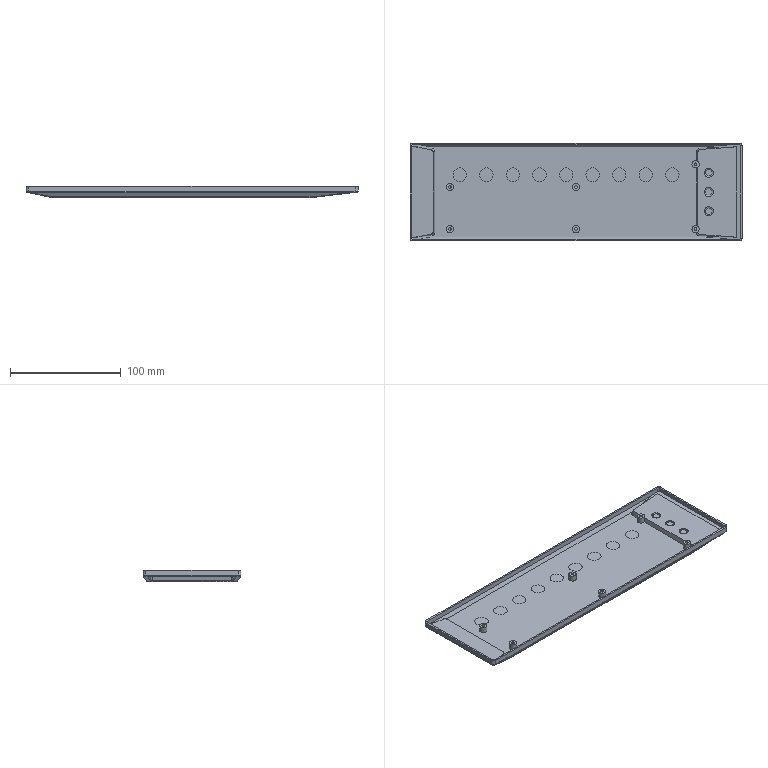NC program | NX | posted with a generic post | part box 300 x 88.5 x 10 mm
Lines 3382 to 4408 of 79950:
(FIXED_CONTOUR_COPY , TOOL : D3R0.5)
N6738 T09 M6
N6740 G54
N6742 G17 G0 G90 X-123.047 Y-18.46 S9500 M3
N6744 G43 Z30. H9
N6746 Z-1.2
N6748 G94 G1 Z-4.25 F1000.
N6750 G2 X-123.197 Y-18.2 R0.3
N6752 G1 Y-18.011 Z-4.267 F2500.
N6754 Y-17.674 Z-4.286
N6756 Y-17.336
N6758 Y-16.998 Z-4.267
N6760 Y-16.799 Z-4.25
N6762 X-123.161 Y-16.634 Z-4.246
N6764 Y-16.806 Z-4.269
N6766 Y-17.041 Z-4.288
N6768 Y-17.336 Z-4.305
N6770 Y-17.674
N6772 Y-18.011 Z-4.285
N6774 Y-18.238 Z-4.264
N6776 Y-18.367 Z-4.246
N6778 X-123.126 Y-18.498 Z-4.243
N6780 X-123.116 Y-18.526 Z-4.244
N6782 Y-18.256 Z-4.283
N6784 Y-18.167 Z-4.294
N6786 Y-17.923 Z-4.313
N6788 Y-17.674 Z-4.328
N6790 Y-17.336
N6792 Y-16.998 Z-4.308
N6794 Y-16.836 Z-4.294
N6796 Y-16.66 Z-4.272
N6798 Y-16.475 Z-4.244
N6800 X-123.055 Y-16.314 Z-4.248
N6802 Y-16.726 Z-4.31
N6804 Y-16.875 Z-4.328
N6806 Y-16.998 Z-4.338
N6808 Y-17.336 Z-4.358
N6810 Y-17.674
N6812 Y-18.011 Z-4.337
N6814 Y-18.129 Z-4.327
N6816 Y-18.349 Z-4.3
N6818 Y-18.689 Z-4.247
N6820 X-122.992 Y-18.829 Z-4.248
N6822 Y-18.687 Z-4.276
N6824 Y-18.349 Z-4.33
N6826 Y-18.09 Z-4.362
N6828 Y-17.799 Z-4.382
N6830 Y-17.674 Z-4.39
N6832 Y-17.336
N6834 Y-16.998 Z-4.369
N6836 Y-16.916 Z-4.362
N6838 Y-16.66 Z-4.331
N6840 Y-16.322 Z-4.278
N6842 Y-16.172 Z-4.248
N6844 X-122.925 Y-16.026 Z-4.25
N6846 Y-16.322 Z-4.309
N6848 Y-16.653 Z-4.363
N6850 Y-16.998 Z-4.403
N6852 Y-17.336 Z-4.424
N6854 Y-17.674
N6856 Y-18.048 Z-4.399
N6858 Y-18.349 Z-4.362
N6860 Y-18.687 Z-4.307
N6862 Y-18.976 Z-4.249
N6864 X-122.89 Y-19.049 Z-4.248
N6866 X-122.849 Y-19.117
N6868 Y-19.008 Z-4.276
N6870 Y-18.67 Z-4.345
N6872 Y-18.332 Z-4.401
N6874 Y-18.011 Z-4.44
N6876 Y-17.674 Z-4.462
N6878 Y-17.336
N6880 Y-16.998 Z-4.44
N6882 Y-16.66 Z-4.4
N6884 Y-16.322 Z-4.343
N6886 Y-15.984 Z-4.274
N6888 Y-15.879 Z-4.247
N6890 X-122.773 Y-15.748 Z-4.245
N6892 Y-15.984 Z-4.307
N6894 Y-16.078 Z-4.329
N6896 Y-16.416 Z-4.397
N6898 Y-16.66 Z-4.437
N6900 Y-16.998 Z-4.479
N6902 Y-17.336 Z-4.5
N6904 Y-17.674
N6906 Y-18.011 Z-4.478
N6908 Y-18.349 Z-4.436
N6910 Y-18.593 Z-4.395
N6912 Y-18.931 Z-4.327
N6914 Y-19.025 Z-4.304
N6916 Y-19.243 Z-4.248
N6918 X-122.692 Y-19.375 Z-4.247
N6920 Y-19.025 Z-4.339
N6922 Y-18.85 Z-4.381
N6924 Y-18.512 Z-4.448
N6926 Y-18.349 Z-4.475
N6928 Y-18.011 Z-4.518
N6930 Y-17.674 Z-4.541
N6932 Y-17.336
N6934 Y-16.998 Z-4.519
N6936 Y-16.66 Z-4.477
N6938 Y-16.497 Z-4.449
N6940 Y-16.159 Z-4.383
N6942 Y-15.984 Z-4.341
N6944 Y-15.646 Z-4.253
N6946 Y-15.626 Z-4.247
N6948 X-122.665 Y-15.586 Z-4.245
N6950 X-122.606 Y-15.511 Z-4.246
N6952 Y-15.646 Z-4.288
N6954 Y-15.984 Z-4.378
N6956 Y-16.246 Z-4.441
N6958 Y-16.584 Z-4.506
N6960 Y-16.66 Z-4.519
N6962 Y-16.998 Z-4.562
N6964 Y-17.336 Z-4.585
N6966 Y-17.674 Z-4.584
N6968 Y-18.011 Z-4.562
N6970 Y-18.349 Z-4.517
N6972 Y-18.426 Z-4.505
N6974 Y-18.764 Z-4.439
N6976 Y-19.025 Z-4.376
N6978 Y-19.363 Z-4.285
N6980 Y-19.488 Z-4.246
N6982 X-122.519 Y-19.598
N6984 Y-19.352 Z-4.324
N6986 Y-19.014 Z-4.416
N6988 Y-18.676 Z-4.497
N6990 Y-18.338 Z-4.561
N6992 Y-18.007 Z-4.605
N6994 Y-17.674 Z-4.628
N6996 Y-17.336
N6998 Y-16.998 Z-4.606
N7000 Y-16.66 Z-4.561
N7002 Y-16.322 Z-4.497
N7004 Y-15.984 Z-4.416
N7006 Y-15.657 Z-4.327
N7008 Y-15.401 Z-4.246
N7010 X-122.43 Y-15.291 Z-4.244
N7012 Y-15.746 Z-4.389
N7014 Y-16.084 Z-4.48
N7016 Y-16.322 Z-4.537
N7018 Y-16.422 Z-4.557
N7020 Y-16.66 Z-4.602
N7022 Y-16.998 Z-4.649
N7024 Y-17.336 Z-4.672
N7026 Y-17.674
N7028 Y-17.968 Z-4.652
N7030 Y-18.25 Z-4.616
N7032 Y-18.349 Z-4.601
N7034 Y-18.588 Z-4.555
N7036 Y-18.687 Z-4.535
N7038 Y-18.926 Z-4.477
N7040 Y-19.263 Z-4.386
N7042 Y-19.708 Z-4.245
N7044 X-122.402 Y-19.741 Z-4.243
N7046 X-122.341 Y-19.799 Z-4.244
N7048 Y-19.568 Z-4.325
N7050 Y-19.174 Z-4.449
N7052 Y-18.836 Z-4.539
N7054 Y-18.687 Z-4.575
N7056 Y-18.499 Z-4.614
N7058 Y-18.349 Z-4.643
N7060 Y-18.161 Z-4.671
N7062 Y-18.011 Z-4.691
N7064 Y-17.929 Z-4.7
N7066 Y-17.674 Z-4.716
N7068 Y-17.585 Z-4.718
N7070 Y-17.336 Z-4.717
N7072 Y-17.101 Z-4.702
N7074 Y-16.998 Z-4.692
N7076 Y-16.849 Z-4.672
N7078 Y-16.66 Z-4.644
N7080 Y-16.511 Z-4.616
N7082 Y-16.322 Z-4.577
N7084 Y-16.173 Z-4.541
N7086 Y-15.835 Z-4.451
N7088 Y-15.448 Z-4.33
N7090 Y-15.308 Z-4.282
N7092 Y-15.201 Z-4.244
N7094 X-122.252 Y-15.118 Z-4.245
N7096 Y-15.308 Z-4.314
N7098 Y-15.566 Z-4.402
N7100 Y-15.924 Z-4.514
N7102 Y-16.322 Z-4.617
N7104 Y-16.66 Z-4.686
N7106 Y-16.998 Z-4.735
N7108 Y-17.149 Z-4.749
N7110 Y-17.336 Z-4.761
N7112 Y-17.543 Z-4.763
N7114 Y-17.674 Z-4.761
N7116 Y-17.89 Z-4.747
N7118 Y-18.011 Z-4.734
N7120 Y-18.349 Z-4.684
N7122 Y-18.687 Z-4.615
N7124 Y-19.085 Z-4.511
N7126 Y-19.445 Z-4.398
N7128 Y-19.701 Z-4.311
N7130 Y-19.882 Z-4.245
N7132 X-122.163 Y-19.966 Z-4.246
N7134 Y-19.672 Z-4.353
N7136 Y-19.334 Z-4.469
N7138 Y-18.996 Z-4.574
N7140 Y-18.673 Z-4.658
N7142 Y-18.335 Z-4.729
N7144 Y-18.011 Z-4.777
N7146 Y-17.856 Z-4.793
N7148 Y-17.674 Z-4.805
N7150 Y-17.512 Z-4.808
N7152 Y-17.336 Z-4.805
N7154 Y-17.184 Z-4.796
N7156 Y-16.998 Z-4.779
N7158 Y-16.66 Z-4.728
N7160 Y-16.337 Z-4.66
N7162 Y-15.984 Z-4.568
N7164 Y-15.646 Z-4.462
N7166 Y-15.338 Z-4.357
N7168 Y-15.035 Z-4.246
N7170 X-122.087 Y-14.965
N7172 X-122.074 Y-14.955
N7174 Y-15.147 Z-4.318
N7176 Y-15.427 Z-4.42
N7178 Y-15.765 Z-4.535
N7180 Y-15.984 Z-4.603
N7182 Y-16.103 Z-4.638
N7184 Y-16.383 Z-4.711
N7186 Y-16.714 Z-4.78
N7188 Y-16.998 Z-4.822
N7190 Y-17.192 Z-4.841
N7192 Y-17.336 Z-4.85
N7194 Y-17.505 Z-4.853
N7196 Y-17.674 Z-4.849
N7198 Y-17.835 Z-4.84
N7200 Y-18.011 Z-4.821
N7202 Y-18.292 Z-4.778
N7204 Y-18.628 Z-4.708
N7206 Y-18.907 Z-4.635
N7208 Y-19.025 Z-4.6
N7210 Y-19.244 Z-4.532
N7212 Y-19.582 Z-4.417
N7214 Y-20.047 Z-4.246
N7216 X-122.02 Y-20.088 Z-4.245
N7218 X-121.985 Y-20.113
N7220 Y-19.888 Z-4.336
N7222 Y-19.493 Z-4.481
N7224 Y-19.155 Z-4.595
N7226 Y-19.025 Z-4.635
N7228 Y-18.817 Z-4.697
N7230 Y-18.584 Z-4.757
N7232 Y-18.249 Z-4.828
N7234 Y-18.011 Z-4.864
N7236 Y-17.791 Z-4.887
N7238 Y-17.674 Z-4.894
N7240 Y-17.498 Z-4.898
N7242 Y-17.336 Z-4.894
N7244 Y-17.178 Z-4.884
N7246 Y-16.998 Z-4.865
N7248 Y-16.755 Z-4.829
N7250 Y-16.429 Z-4.761
N7252 Y-16.192 Z-4.699
N7254 Y-15.984 Z-4.638
N7256 Y-15.854 Z-4.598
N7258 Y-15.516 Z-4.484
N7260 Y-15.127 Z-4.341
N7262 Y-14.887 Z-4.244
N7264 X-121.894 Y-14.825 Z-4.246
N7266 Y-15.279 Z-4.428
N7268 Y-15.646 Z-4.562
N7270 Y-15.984 Z-4.674
N7272 Y-16.283 Z-4.761
N7274 Y-16.475 Z-4.812
N7276 Y-16.66 Z-4.851
N7278 Y-16.796 Z-4.878
N7280 Y-16.943 Z-4.9
N7282 X-121.803 Y-16.703
N7284 Y-16.694
N7286 Y-16.526 Z-4.864
N7288 Y-16.322 Z-4.81
N7290 Y-15.998 Z-4.714
N7292 Y-15.698 Z-4.614
N7294 Y-15.36 Z-4.489
N7296 Y-14.821 Z-4.271
N7298 Y-14.764 Z-4.246
N7300 X-121.729 Y-14.716 Z-4.245
N7302 X-121.711 Y-14.705
N7304 Y-14.87 Z-4.317
N7306 Y-15.453 Z-4.555
N7308 Y-15.79 Z-4.679
N7310 Y-16.023 Z-4.758
N7312 Y-16.167 Z-4.804
N7314 Y-16.322 Z-4.849
N7316 Y-16.517 Z-4.9
N7318 X-121.618 Y-16.377
N7320 Y-16.368
N7322 Y-16.285 Z-4.877
N7324 Y-16.048 Z-4.801
N7326 Y-15.883 Z-4.745
N7328 Y-15.545 Z-4.62
N7330 Y-15.207 Z-4.483
N7332 Y-14.918 Z-4.363
N7334 Y-14.653 Z-4.248
N7336 X-121.525 Y-14.601 Z-4.247
N7338 Y-14.967 Z-4.41
N7340 Y-15.301 Z-4.549
N7342 Y-15.639 Z-4.687
N7344 Y-15.984 Z-4.814
N7346 Y-16.073 Z-4.846
N7348 Y-16.245 Z-4.9
N7350 X-121.431 Y-16.136
N7352 Y-16.132
N7354 Y-15.714 Z-4.746
N7356 Y-15.396 Z-4.615
N7358 Y-15.058 Z-4.473
N7360 Y-14.603 Z-4.269
N7362 Y-14.55 Z-4.244
N7364 X-121.394 Y-14.531 Z-4.243
N7366 X-121.335 Y-14.508 Z-4.245
N7368 Y-14.815 Z-4.387
N7370 Y-15.153 Z-4.538
N7372 Y-15.308 Z-4.602
N7374 Y-15.491 Z-4.682
N7376 Y-15.788 Z-4.804
N7378 Y-16.042 Z-4.9
N7380 X-121.24 Y-15.958
N7382 Y-15.863 Z-4.863
N7384 Y-15.587 Z-4.749
N7386 Y-15.249 Z-4.603
N7388 Y-14.911 Z-4.452
N7390 Y-14.471 Z-4.248
N7392 X-121.143 Y-14.434 Z-4.249
N7394 Y-14.67 Z-4.36
N7396 Y-15.008 Z-4.517
N7398 Y-15.382 Z-4.685
N7400 Y-15.666 Z-4.809
N7402 Y-15.886 Z-4.9
N7404 X-121.046 Y-15.82 Z-4.898
N7406 Y-15.574 Z-4.794
N7408 Y-15.105 Z-4.581
N7410 Y-14.516 Z-4.304
N7412 Y-14.399 Z-4.248
N7414 X-120.949 Y-14.371 Z-4.25
N7416 Y-14.864 Z-4.486
N7418 Y-15.202 Z-4.645
N7420 Y-15.763 Z-4.9
N7422 Y-15.771
N7424 X-120.851 Y-15.723
N7426 Y-15.712
N7428 Y-15.3 Z-4.709
N7430 Y-14.342 Z-4.252
N7432 X-120.752 Y-14.316 Z-4.25
N7434 Y-14.723 Z-4.448
N7436 Y-15.509 Z-4.825
N7438 Y-15.671 Z-4.9
N7440 Y-15.675
N7442 X-120.698 Y-15.649
N7444 X-120.654 Y-15.635
N7446 Y-15.16 Z-4.672
N7448 Y-14.294 Z-4.249
N7450 X-120.555 Y-14.276 Z-4.251
N7452 Y-15.603 Z-4.9
N7454 X-120.499 Y-15.586
N7456 X-120.455 Y-15.576
N7458 Y-15.093 Z-4.663
N7460 Y-14.582 Z-4.408
N7462 Y-14.26 Z-4.25
N7464 X-120.356 Y-14.244 Z-4.247
N7466 Y-15.121 Z-4.682
N7468 Y-15.358 Z-4.803
N7470 Y-15.555 Z-4.9
N7472 X-120.256 Y-15.545
N7474 Y-15.54
N7476 Y-14.382 Z-4.319
N7478 Y-14.238 Z-4.248
N7480 X-120.157 Y-14.231 Z-4.249
N7482 Y-15.532 Z-4.9
N7484 Y-15.536
N7486 X-120.057 Y-15.526
N7488 Y-15.194 Z-4.735
N7490 Y-14.97 Z-4.619
N7492 Y-14.226 Z-4.246
N7494 X-120.007 Y-14.224 Z-4.245
N7496 X-119.957 Y-14.226 Z-4.246
N7498 Y-14.97 Z-4.619
N7500 Y-15.222 Z-4.749
N7502 Y-15.521 Z-4.898
N7504 X-119.857 Y-15.52 Z-4.895
N7506 Y-14.231 Z-4.249
N7508 X-119.757 Y-14.237 Z-4.248
N7510 Y-15.308 Z-4.784
N7512 Y-15.535 Z-4.898
N7514 X-119.657 Y-15.552 Z-4.9
N7516 Y-15.308 Z-4.78
N7518 Y-14.97 Z-4.608
N7520 Y-14.244 Z-4.247
N7522 X-119.558 Y-14.259 Z-4.25
N7524 Y-15.034 Z-4.633
N7526 Y-15.308 Z-4.77
N7528 Y-15.573 Z-4.9
N7530 X-119.458 Y-15.597 Z-4.899
N7532 Y-14.274 Z-4.251
N7534 X-119.359 Y-14.291 Z-4.249
N7536 Y-14.835 Z-4.516
N7538 Y-15.628 Z-4.899
N7540 X-119.31 Y-15.647 Z-4.9
N7542 X-119.26 Y-15.67
N7544 Y-15.666
N7546 Y-15.394 Z-4.771
N7548 Y-14.419 Z-4.302
N7550 Y-14.313 Z-4.25
N7552 X-119.162 Y-14.339 Z-4.252
N7554 Y-15.312 Z-4.717
N7556 Y-15.706 Z-4.9
N7558 Y-15.717
N7560 X-119.064 Y-15.763
N7562 Y-15.756
N7564 Y-15.215 Z-4.653
N7566 Y-14.579 Z-4.352
N7568 Y-14.366 Z-4.25
N7570 X-118.966 Y-14.394 Z-4.248
N7572 Y-14.779 Z-4.431
N7574 Y-15.117 Z-4.589
N7576 Y-15.646 Z-4.828
N7578 Y-15.812 Z-4.898
N7580 X-118.869 Y-15.877 Z-4.9
N7582 Y-15.672 Z-4.815
N7584 Y-15.406 Z-4.699
N7586 Y-14.97 Z-4.501
N7588 Y-14.467 Z-4.267
N7590 Y-14.429 Z-4.249
N7592 X-118.772 Y-14.466 Z-4.248
N7594 Y-14.923 Z-4.46
N7596 Y-15.308 Z-4.631
N7598 Y-15.646 Z-4.777
N7600 Y-15.872 Z-4.871
N7602 Y-15.947 Z-4.9
N7604 X-118.677 Y-16.031
N7606 Y-15.798 Z-4.812
N7608 Y-15.503 Z-4.691
N7610 Y-15.308 Z-4.606
N7612 Y-15.165 Z-4.546
N7614 Y-14.827 Z-4.395
N7616 Y-14.502 Z-4.245
N7618 X-118.624 Y-14.522 Z-4.243
N7620 X-118.583 Y-14.544 Z-4.244
N7622 Y-14.733 Z-4.331
N7624 Y-15.071 Z-4.482
N7626 Y-15.308 Z-4.581
N7628 Y-15.409 Z-4.625
N7630 Y-15.785 Z-4.777
N7632 Y-16.119 Z-4.9
N7634 Y-16.123
N7636 X-118.49 Y-16.229
N7638 Y-16.072 Z-4.85
N7640 Y-15.652 Z-4.697
N7642 Y-15.308 Z-4.556
N7644 Y-14.978 Z-4.419
N7646 Y-14.593 Z-4.247
N7648 X-118.4 Y-14.642 Z-4.248
N7650 Y-14.97 Z-4.39
N7652 Y-15.308 Z-4.529
N7654 Y-15.564 Z-4.634
N7656 Y-15.902 Z-4.758
N7658 Y-16.052 Z-4.81
N7660 Y-16.338 Z-4.9
N7662 Y-16.342
N7664 X-118.357 Y-16.403 Z-4.899
N7666 X-118.311 Y-16.478
N7668 Y-16.322 Z-4.858
N7670 Y-16.196 Z-4.821
N7672 Y-15.984 Z-4.752
N7674 Y-15.813 Z-4.695
N7676 Y-15.475 Z-4.57
N7678 Y-14.881 Z-4.328
N7680 Y-14.692 Z-4.245
N7682 X-118.278 Y-14.71
N7684 X-118.227 Y-14.745 Z-4.246
N7686 Y-14.837 Z-4.286
N7688 Y-15.39 Z-4.51
N7690 Y-15.728 Z-4.635
N7692 Y-16.088 Z-4.754
N7694 Y-16.322 Z-4.823
N7696 Y-16.527 Z-4.877
N7698 Y-16.625 Z-4.899
N7700 X-118.159 Y-16.803 Z-4.9
N7702 Y-16.782
N7704 Y-16.66 Z-4.876
N7706 Y-16.495 Z-4.839
N7708 Y-16.322 Z-4.794
N7710 Y-15.984 Z-4.695
N7712 Y-15.66 Z-4.587
N7714 Y-15.322 Z-4.462
N7716 Y-14.791 Z-4.247
N7718 X-118.094 Y-14.836
N7720 Y-15.235 Z-4.408
N7722 Y-15.646 Z-4.557
N7724 Y-15.984 Z-4.669
N7726 Y-16.27 Z-4.753
N7728 Y-16.463 Z-4.803
N7730 Y-16.66 Z-4.846
N7732 Y-16.79 Z-4.872
N7734 Y-16.978 Z-4.9
N7736 X-118.057 Y-17.171
N7738 Y-17.136
N7740 Y-16.998 Z-4.885
N7742 Y-16.774 Z-4.852
N7744 Y-16.572 Z-4.811
N7746 Y-16.445 Z-4.783
N7748 Y-16.234 Z-4.728
N7750 Y-15.896 Z-4.627
N7752 Y-15.558 Z-4.514
N7754 Y-15.185 Z-4.377
N7756 Y-14.862 Z-4.246
N7758 X-118.053 Y-14.828
N7760 X-118.07 Y-14.798
N7762 X-118.102 Y-14.784
N7764 Z-1.096
N7766 G0 Z-0.496
N7768 X-121.662 Y-16.753
N7770 Z-1.096
N7772 G1 Z-4.9 F1000.
N7774 G3 X-121.894 Y-16.943 R0.3
N7776 G1 X-121.907 Y-16.981 F2500.
N7778 X-121.971 Y-17.318
N7780 X-121.972 Y-17.67
N7782 X-121.91 Y-18.011
N7784 X-121.894 Y-18.053
N7786 Y-18.205 Z-4.878
N7788 Y-18.349 Z-4.85
N7790 Y-18.539 Z-4.808
N7792 Y-18.727 Z-4.759
N7794 Y-19.065 Z-4.659
N7796 Y-19.403 Z-4.545
N7798 Y-19.758 Z-4.414
N7800 Y-20.174 Z-4.246
N7802 X-121.803 Y-20.236
N7804 Y-19.987 Z-4.349
N7806 Y-19.649 Z-4.486
N7808 Y-19.311 Z-4.61
N7810 Y-18.961 Z-4.727
N7812 Y-18.687 Z-4.808
N7814 Y-18.495 Z-4.858
N7816 Y-18.306 Z-4.9
N7818 Y-18.298
N7820 X-121.782 Y-18.357
N7822 X-121.763 Y-18.398 Z-4.898
N7824 X-121.711 Y-18.483 Z-4.9
N7826 Y-18.687 Z-4.846
N7828 Y-18.847 Z-4.799
N7830 Y-19.025 Z-4.741
N7832 Y-19.219 Z-4.676
N7834 Y-19.557 Z-4.551
N7836 Y-20.134 Z-4.315
N7838 Y-20.295 Z-4.245
N7840 X-121.618 Y-20.348 Z-4.246
N7842 Y-20.039 Z-4.381
N7844 Y-19.701 Z-4.52
N7846 Y-19.464 Z-4.617
N7848 Y-19.126 Z-4.742
N7850 Y-18.953 Z-4.801
N7852 Y-18.687 Z-4.885
N7854 Y-18.627 Z-4.9
N7856 X-121.569 Y-18.703
N7858 X-121.525 Y-18.757
N7860 Y-18.925 Z-4.846
N7862 Y-19.032 Z-4.809
N7864 Y-19.37 Z-4.684
N7866 Y-20.039 Z-4.407
N7868 Y-20.402 Z-4.246
N7870 X-121.466 Y-20.434 Z-4.244
N7872 X-121.431 Y-20.451
N7874 Y-20.039 Z-4.43
N7876 Y-19.952 Z-4.469
N7878 Y-19.614 Z-4.612
N7880 Y-19.248 Z-4.761
N7882 Y-18.866 Z-4.9
N7884 X-121.394 Y-18.905 Z-4.899
N7886 X-121.335 Y-18.958
N7888 Y-19.216 Z-4.803
N7890 Y-19.518 Z-4.678
N7892 Y-19.701 Z-4.598
N7894 Y-19.856 Z-4.534
N7896 Y-20.194 Z-4.383
N7898 Y-20.491 Z-4.245
N7900 X-121.24 Y-20.529 Z-4.248
N7902 Y-20.039 Z-4.474
N7904 Y-19.76 Z-4.599
N7906 Y-19.363 Z-4.77
N7908 Y-19.139 Z-4.863
N7910 Y-19.044 Z-4.9
N7912 X-121.143 Y-19.116 Z-4.899
N7914 Y-19.342 Z-4.805
N7916 Y-19.701 Z-4.647
N7918 Y-20.039 Z-4.495
N7920 Y-20.566 Z-4.249
N7922 X-121.046 Y-20.601 Z-4.248
N7924 Y-20.242 Z-4.419
N7926 Y-19.904 Z-4.576
N7928 Y-19.363 Z-4.821
N7930 Y-19.18 Z-4.898
N7932 X-120.949 Y-19.229 Z-4.9
N7934 Y-19.237
N7936 Y-19.489 Z-4.785
N7938 Y-19.807 Z-4.641
N7940 Y-20.435 Z-4.344
N7942 Y-20.629 Z-4.25
N7944 X-120.851 Y-20.658 Z-4.252
N7946 Y-19.709 Z-4.705
N7948 Y-19.288 Z-4.9
N7950 Y-19.277
N7952 X-120.752 Y-19.325
N7954 Y-19.328
N7956 Y-19.623 Z-4.761
N7958 Y-20.595 Z-4.294
N7960 Y-20.684 Z-4.25
N7962 X-120.702 Y-20.697 Z-4.249
N7964 X-120.654 Y-20.706
N7966 Y-20.187 Z-4.503
N7968 Y-19.367 Z-4.9
N7970 X-120.576 Y-19.395 Z-4.898
N7972 X-120.555 Y-19.4 Z-4.899
N7974 Y-20.724 Z-4.25
N7976 X-120.506 Y-20.733 Z-4.251
N7978 X-120.455 Y-20.741 Z-4.249
N7980 Y-19.988 Z-4.621
N7982 Y-19.701 Z-4.764
N7984 Y-19.424 Z-4.9
N7986 X-120.356 Y-19.445
N7988 Y-19.701 Z-4.774
N7990 Y-20.039 Z-4.602
N7992 Y-20.757 Z-4.246
N7994 X-120.256 Y-20.766
N7996 Y-19.701 Z-4.779
N7998 Y-19.461 Z-4.9
N8000 Y-19.455
N8002 X-120.157 Y-19.464
N8004 Y-19.468
N8006 Y-20.774 Z-4.246
N8008 X-120.057 Y-20.782 Z-4.243
N8010 Y-20.377 Z-4.445
N8012 Y-20.153 Z-4.561
N8014 Y-19.474 Z-4.899
N8016 X-120.009 Y-19.478 Z-4.898
N8018 X-119.957 Y-19.479
N8020 Y-20.125 Z-4.575
N8022 Y-20.377 Z-4.445
N8024 Y-20.782 Z-4.243
N8026 X-119.857 Y-20.775 Z-4.246
N8028 Y-19.481 Z-4.894
N8030 X-119.757 Y-19.465 Z-4.898
N8032 Y-19.701 Z-4.78
N8034 Y-20.039 Z-4.61
N8036 Y-20.767 Z-4.246
N8038 X-119.657 Y-20.758
N8040 Y-19.875 Z-4.685
N8042 Y-19.716 Z-4.768
N8044 Y-19.448 Z-4.9
N8046 X-119.558 Y-19.426
N8048 Y-19.913 Z-4.661
N8050 Y-20.039 Z-4.597
N8052 Y-20.742 Z-4.249
N8054 X-119.458 Y-20.726 Z-4.251
N8056 Y-19.403 Z-4.899
N8058 X-119.424 Y-19.395 Z-4.898
N8060 X-119.359 Y-19.372 Z-4.9
N8062 Y-20.174 Z-4.511
N8064 Y-20.709 Z-4.249
N8066 X-119.316 Y-20.701 Z-4.248
N8068 X-119.26 Y-20.687 Z-4.25
N8070 Y-20.273 Z-4.451
N8072 Y-19.503 Z-4.821
N8074 Y-19.333 Z-4.9
N8076 Y-19.33
N8078 X-119.162 Y-19.283
N8080 Y-19.294
N8082 Y-19.692 Z-4.715
N8084 Y-20.661 Z-4.252
N8086 X-119.064 Y-20.634 Z-4.25
N8088 Y-20.132 Z-4.49
N8090 Y-19.794 Z-4.649
N8092 Y-19.327 Z-4.863
N8094 Y-19.244 Z-4.9
N8096 Y-19.237
N8098 X-119.006 Y-19.209
N8100 X-118.966 Y-19.188 Z-4.898
N8102 Y-19.363 Z-4.824
N8104 Y-19.554 Z-4.739
N8106 Y-19.701 Z-4.67
N8108 Y-19.892 Z-4.584
N8110 Y-20.476 Z-4.31
N8112 Y-20.606 Z-4.248
N8114 X-118.869 Y-20.57 Z-4.249
N8116 Y-20.327 Z-4.364
N8118 Y-19.989 Z-4.521
N8120 Y-19.588 Z-4.701
N8122 Y-19.336 Z-4.811
N8124 Y-19.122 Z-4.9
N8126 X-118.772 Y-19.054
N8128 Y-19.129 Z-4.87
N8130 Y-19.411 Z-4.754
N8132 Y-19.748 Z-4.607
N8134 Y-20.086 Z-4.456
N8136 Y-20.534 Z-4.248
N8138 X-118.677 Y-20.497 Z-4.245
N8140 Y-20.182 Z-4.391
N8142 Y-19.844 Z-4.542
N8144 Y-19.701 Z-4.602
N8146 Y-19.506 Z-4.687
N8148 Y-19.206 Z-4.811
N8150 Y-18.97 Z-4.9
N8152 X-118.616 Y-18.914
N8154 X-118.583 Y-18.876
N8156 Y-18.882
N8158 Y-19.282 Z-4.752
N8160 Y-19.6 Z-4.621
N8162 Y-19.701 Z-4.577
N8164 Y-19.938 Z-4.478
N8166 Y-20.395 Z-4.273
N8168 Y-20.455 Z-4.245
N8170 X-118.49 Y-20.406 Z-4.248
N8172 Y-20.031 Z-4.414
N8174 Y-19.694 Z-4.556
N8176 Y-19.353 Z-4.695
N8178 Y-18.93 Z-4.85
N8180 Y-18.774 Z-4.9
N8182 Y-18.77
N8184 X-118.431 Y-18.703
N8186 X-118.4 Y-18.656
N8188 Y-18.71 Z-4.886
N8190 Y-18.959 Z-4.806
N8192 Y-19.108 Z-4.755
N8194 Y-19.446 Z-4.63
N8196 Y-19.783 Z-4.492
N8198 Y-20.078 Z-4.37
N8200 Y-20.358 Z-4.247
N8202 X-118.311 Y-20.308 Z-4.245
N8204 Y-20.121 Z-4.327
N8206 Y-19.535 Z-4.567
N8208 Y-19.197 Z-4.692
N8210 Y-18.982 Z-4.765
N8212 Y-18.82 Z-4.816
N8214 Y-18.687 Z-4.855
N8216 Y-18.519 Z-4.9
N8218 X-118.272 Y-18.458
N8220 X-118.227 Y-18.373
N8222 Y-18.462 Z-4.88
N8224 Y-18.687 Z-4.82
N8226 Y-18.924 Z-4.751
N8228 Y-19.281 Z-4.632
N8230 Y-19.619 Z-4.507
N8232 Y-20.165 Z-4.285
N8234 Y-20.255 Z-4.245
N8236 X-118.159 Y-20.21 Z-4.247
N8238 Y-19.687 Z-4.459
N8240 Y-19.349 Z-4.583
N8242 Y-19.008 Z-4.697
N8244 Y-18.687 Z-4.792
N8246 Y-18.505 Z-4.839
N8248 Y-18.349 Z-4.874
N8250 Y-18.218 Z-4.9
N8252 Y-18.196
N8254 X-118.094 Y-18.02
N8256 Y-18.211 Z-4.871
N8258 Y-18.349 Z-4.844
N8260 Y-18.54 Z-4.802
N8262 Y-18.739 Z-4.751
N8264 Y-19.077 Z-4.65
N8266 Y-19.415 Z-4.537
N8268 Y-19.776 Z-4.404
N8270 Y-20.164 Z-4.247
N8272 X-118.057 Y-20.139 Z-4.246
N8274 Y-19.829 Z-4.371
N8276 Y-19.451 Z-4.51
N8278 Y-19.113 Z-4.624
N8280 Y-18.776 Z-4.725
N8282 Y-18.559 Z-4.782
N8284 Y-18.349 Z-4.827
N8286 Y-18.229 Z-4.851
N8288 Y-17.986 Z-4.886
N8290 Y-17.866 Z-4.9
N8292 Y-17.829
N8294 X-118.059 Y-17.784
N8296 X-118.036 Y-17.745
N8298 X-117.997 Y-17.725
N8300 Z-1.096
N8302 G0 Z-0.496
N8304 X-118.095 Y-20.22
N8306 Z-1.096
N8308 G1 Z-4.246 F1000.
N8310 X-118.102 Y-20.187
N8312 X-118.087 Y-20.155
N8314 X-118.057 Y-20.139
N8316 X-117.967 Y-20.077 Z-4.245 F2500.
N8318 Y-19.96 Z-4.293
N8320 Y-19.541 Z-4.446
N8322 Y-19.203 Z-4.561
N8324 Y-19.025 Z-4.617
N8326 Y-18.865 Z-4.664
N8328 Y-18.605 Z-4.731
N8330 Y-18.272 Z-4.801
N8332 Y-18.011 Z-4.84
N8334 Y-17.814 Z-4.861
N8336 Y-17.674 Z-4.87
N8338 Y-17.512 Z-4.874
N8340 Y-17.336 Z-4.87
N8342 Y-17.195 Z-4.862
N8344 Y-16.998 Z-4.842
N8346 Y-16.733 Z-4.802
N8348 Y-16.4 Z-4.733
N8350 Y-16.144 Z-4.666
N8352 Y-15.984 Z-4.619
N8354 Y-15.806 Z-4.564
N8356 Y-15.468 Z-4.45
N8358 Y-15.06 Z-4.3
N8360 Y-14.924 Z-4.245
N8362 X-117.925 Y-14.955
N8364 X-117.878 Y-14.997 Z-4.246
N8366 Y-15.379 Z-4.386
N8368 Y-15.716 Z-4.501
N8370 Y-16.054 Z-4.604
N8372 Y-16.392 Z-4.691
N8374 Y-16.692 Z-4.753
N8376 Y-16.998 Z-4.798
N8378 Y-17.188 Z-4.817
N8380 Y-17.336 Z-4.826
N8382 Y-17.52 Z-4.829
N8384 Y-17.674 Z-4.825
N8386 Y-17.822 Z-4.816
N8388 Y-18.011 Z-4.797
N8390 Y-18.315 Z-4.751
N8392 Y-18.651 Z-4.681
N8394 Y-18.955 Z-4.602
N8396 Y-19.293 Z-4.498
N8398 Y-19.631 Z-4.383
N8400 Y-20.003 Z-4.246
N8402 X-117.789 Y-19.92
N8404 Y-19.701 Z-4.326
N8406 Y-19.389 Z-4.432
N8408 Y-19.025 Z-4.545
N8410 Y-18.687 Z-4.633
N8412 Y-18.349 Z-4.703
N8414 Y-18.011 Z-4.754
N8416 Y-17.839 Z-4.771
N8418 Y-17.674 Z-4.781
N8420 Y-17.516 Z-4.784
N8422 Y-17.317 Z-4.78
N8424 Y-17.172 Z-4.771
N8426 Y-16.979 Z-4.753
N8428 Y-16.641 Z-4.702
N8430 Y-16.303 Z-4.631
N8432 Y-15.965 Z-4.543
N8434 Y-15.62 Z-4.435
N8436 Y-15.308 Z-4.329
N8438 Y-15.08 Z-4.246
N8440 X-117.699 Y-15.163 Z-4.244
N8442 Y-15.306 Z-4.296
N8444 Y-15.501 Z-4.362
N8446 Y-15.875 Z-4.48
N8448 Y-16.213 Z-4.569
N8450 Y-16.322 Z-4.595
N8452 Y-16.551 Z-4.643
N8454 Y-16.66 Z-4.663
N8456 Y-16.998 Z-4.712
N8458 Y-17.123 Z-4.723
N8460 Y-17.336 Z-4.737
N8462 Y-17.574 Z-4.738
N8464 Y-17.674 Z-4.736
N8466 Y-17.887 Z-4.723
N8468 Y-18.011 Z-4.711
N8470 Y-18.349 Z-4.662
N8472 Y-18.458 Z-4.641
N8474 Y-18.687 Z-4.593
N8476 Y-18.796 Z-4.567
N8478 Y-19.134 Z-4.477
N8480 Y-19.512 Z-4.358
N8482 Y-19.701 Z-4.294
N8484 Y-19.837 Z-4.244
N8486 X-117.61 Y-19.754 Z-4.243
N8488 Y-19.635 Z-4.285
N8490 Y-19.223 Z-4.414
N8492 Y-18.885 Z-4.505
N8494 Y-18.687 Z-4.553
N8496 Y-18.547 Z-4.582
N8498 Y-18.349 Z-4.62
N8500 Y-18.21 Z-4.641
N8502 Y-18.011 Z-4.667
N8504 Y-17.872 Z-4.679
N8506 Y-17.674 Z-4.692
N8508 Y-17.336
N8510 Y-17.074 Z-4.675
N8512 Y-16.998 Z-4.668
N8514 Y-16.8 Z-4.642
N8516 Y-16.66 Z-4.621
N8518 Y-16.462 Z-4.584
N8520 Y-16.322 Z-4.555
N8522 Y-16.124 Z-4.508
N8524 Y-15.786 Z-4.417
N8526 Y-15.381 Z-4.29
N8528 Y-15.247 Z-4.243
N8530 X-117.567 Y-15.294 Z-4.245
N8532 X-117.521 Y-15.352 Z-4.246
N8534 Y-15.697 Z-4.354
N8536 Y-16.034 Z-4.446
N8538 Y-16.322 Z-4.514
N8540 Y-16.66 Z-4.579
N8542 Y-17.025 Z-4.627
N8544 Y-17.336 Z-4.648
N8546 Y-17.674
N8548 Y-18.011 Z-4.624
N8550 Y-18.349 Z-4.578
N8552 Y-18.687 Z-4.512
N8554 Y-19.025 Z-4.43
N8556 Y-19.313 Z-4.351
N8558 Y-19.648 Z-4.246
N8560 X-117.431 Y-19.536
N8562 Y-19.362 Z-4.301
N8564 Y-19.025 Z-4.392
N8566 Y-18.687 Z-4.472
N8568 Y-18.349 Z-4.535
N8570 Y-18.011 Z-4.58
N8572 Y-17.674 Z-4.603
N8574 Y-17.336
N8576 Y-16.998 Z-4.581
N8578 Y-16.66 Z-4.537
N8580 Y-16.283 Z-4.466
N8582 Y-15.984 Z-4.394
N8584 Y-15.646 Z-4.303
N8586 Y-15.464 Z-4.246
N8588 X-117.342 Y-15.576 Z-4.245
N8590 Y-15.646 Z-4.267
N8592 Y-15.984 Z-4.356
N8594 Y-16.194 Z-4.406
N8596 Y-16.531 Z-4.472
N8598 Y-16.66 Z-4.493
N8600 Y-16.998 Z-4.536
N8602 Y-17.336 Z-4.558
N8604 Y-17.674
N8606 Y-18.011 Z-4.536
N8608 Y-18.349 Z-4.492
N8610 Y-18.478 Z-4.47
N8612 Y-18.816 Z-4.404
N8614 Y-19.025 Z-4.354
N8616 Y-19.363 Z-4.264
N8618 Y-19.424 Z-4.245
N8620 X-117.32 Y-19.395
N8622 X-117.296 Y-19.358 Z-4.247
N8624 X-117.253 Y-19.286
N8626 Y-19.025 Z-4.315
N8628 Y-18.905 Z-4.344
N8630 Y-18.567 Z-4.412
N8632 Y-18.349 Z-4.449
N8634 Y-18.011 Z-4.491
N8636 Y-17.674 Z-4.513
N8638 Y-17.336
N8640 Y-16.998 Z-4.492
N8642 Y-16.66 Z-4.45
N8644 Y-16.442 Z-4.414
N8646 Y-16.104 Z-4.346
N8648 Y-15.984 Z-4.318
N8650 Y-15.707 Z-4.246
N8652 X-117.238 Y-15.73 Z-4.245
N8654 X-117.164 Y-15.858 Z-4.247
N8656 Y-16.015 Z-4.287
N8658 Y-16.353 Z-4.355
N8660 Y-16.69 Z-4.411
N8662 Y-16.998 Z-4.447
N8664 Y-17.336 Z-4.468
N8666 Y-17.674
N8668 Y-18.011 Z-4.446
N8670 Y-18.349 Z-4.405
N8672 Y-18.687 Z-4.348
N8674 Y-19.025 Z-4.277
N8676 Y-19.138 Z-4.248
N8678 X-117.11 Y-19.049
N8680 X-117.074 Y-18.974 Z-4.249
N8682 Y-18.687 Z-4.307
N8684 Y-18.349 Z-4.362
N8686 Y-18.011 Z-4.402
N8688 Y-17.674 Z-4.423
N8690 Y-17.336
N8692 Y-16.957 Z-4.399
N8694 Y-16.653 Z-4.362
N8696 Y-16.322 Z-4.309
N8698 Y-16.026 Z-4.249
N8700 X-116.985 Y-16.215 Z-4.246
N8702 Y-16.322 Z-4.268
N8704 Y-16.712 Z-4.327
N8706 Y-16.901 Z-4.35
N8708 Y-16.998 Z-4.358
N8710 Y-17.336 Z-4.378
N8712 Y-17.674
N8714 Y-18.011 Z-4.357
N8716 Y-18.104 Z-4.349
N8718 Y-18.349 Z-4.319
N8720 Y-18.685 Z-4.266
N8722 Y-18.782 Z-4.247
N8724 X-116.941 Y-18.685 Z-4.246
N8726 X-116.896 Y-18.57 Z-4.243
N8728 Y-18.26 Z-4.288
N8730 Y-18.16 Z-4.3
N8732 Y-17.911 Z-4.319
N8734 Y-17.674 Z-4.333
N8736 Y-17.336
N8738 Y-16.998 Z-4.313
N8740 Y-16.843 Z-4.3
N8742 Y-16.66 Z-4.277
N8744 Y-16.429 Z-4.242
N8746 X-116.842 Y-16.625 Z-4.246
N8748 X-116.806 Y-16.783 Z-4.251
N8750 Y-16.998 Z-4.269
N8752 Y-17.336 Z-4.288
N8754 Y-17.674
N8756 Y-18.011 Z-4.268
N8758 Y-18.216 Z-4.251
N8760 X-116.807 Y-18.251
N8762 X-116.776 Y-18.268
N8764 Z-0.6
N8766 G0 Z30.
N8768 X-120.749 Y3.229
N8770 Z-0.6
N8772 G1 Z-4.248 F1000.
N8774 X-120.732 Y3.198
N8776 X-120.697 Y3.199
N8778 X-120.506 Z-4.268 F2500.
N8780 X-120.169 Z-4.284
N8782 X-119.831
N8784 X-119.494 Z-4.268